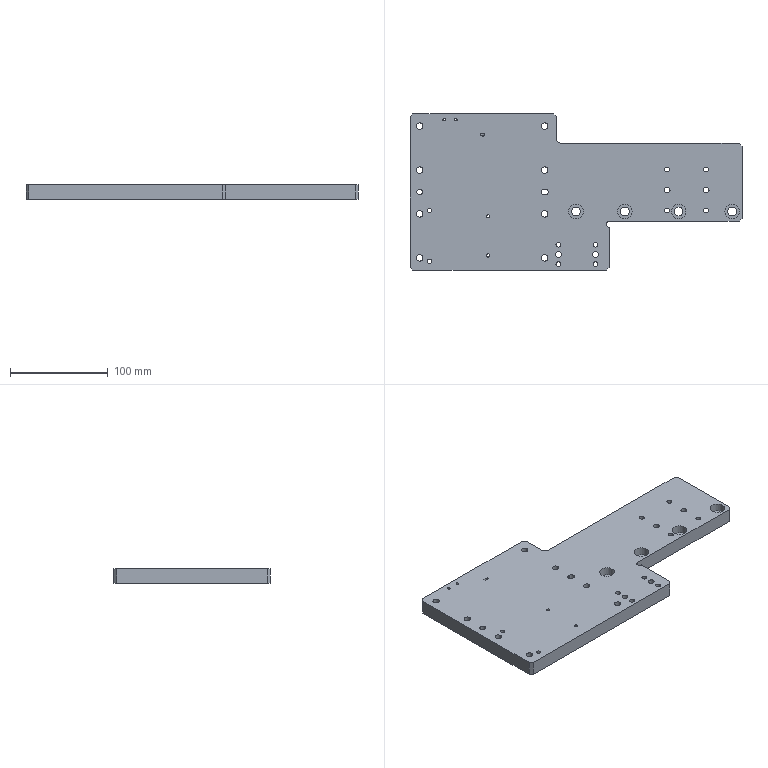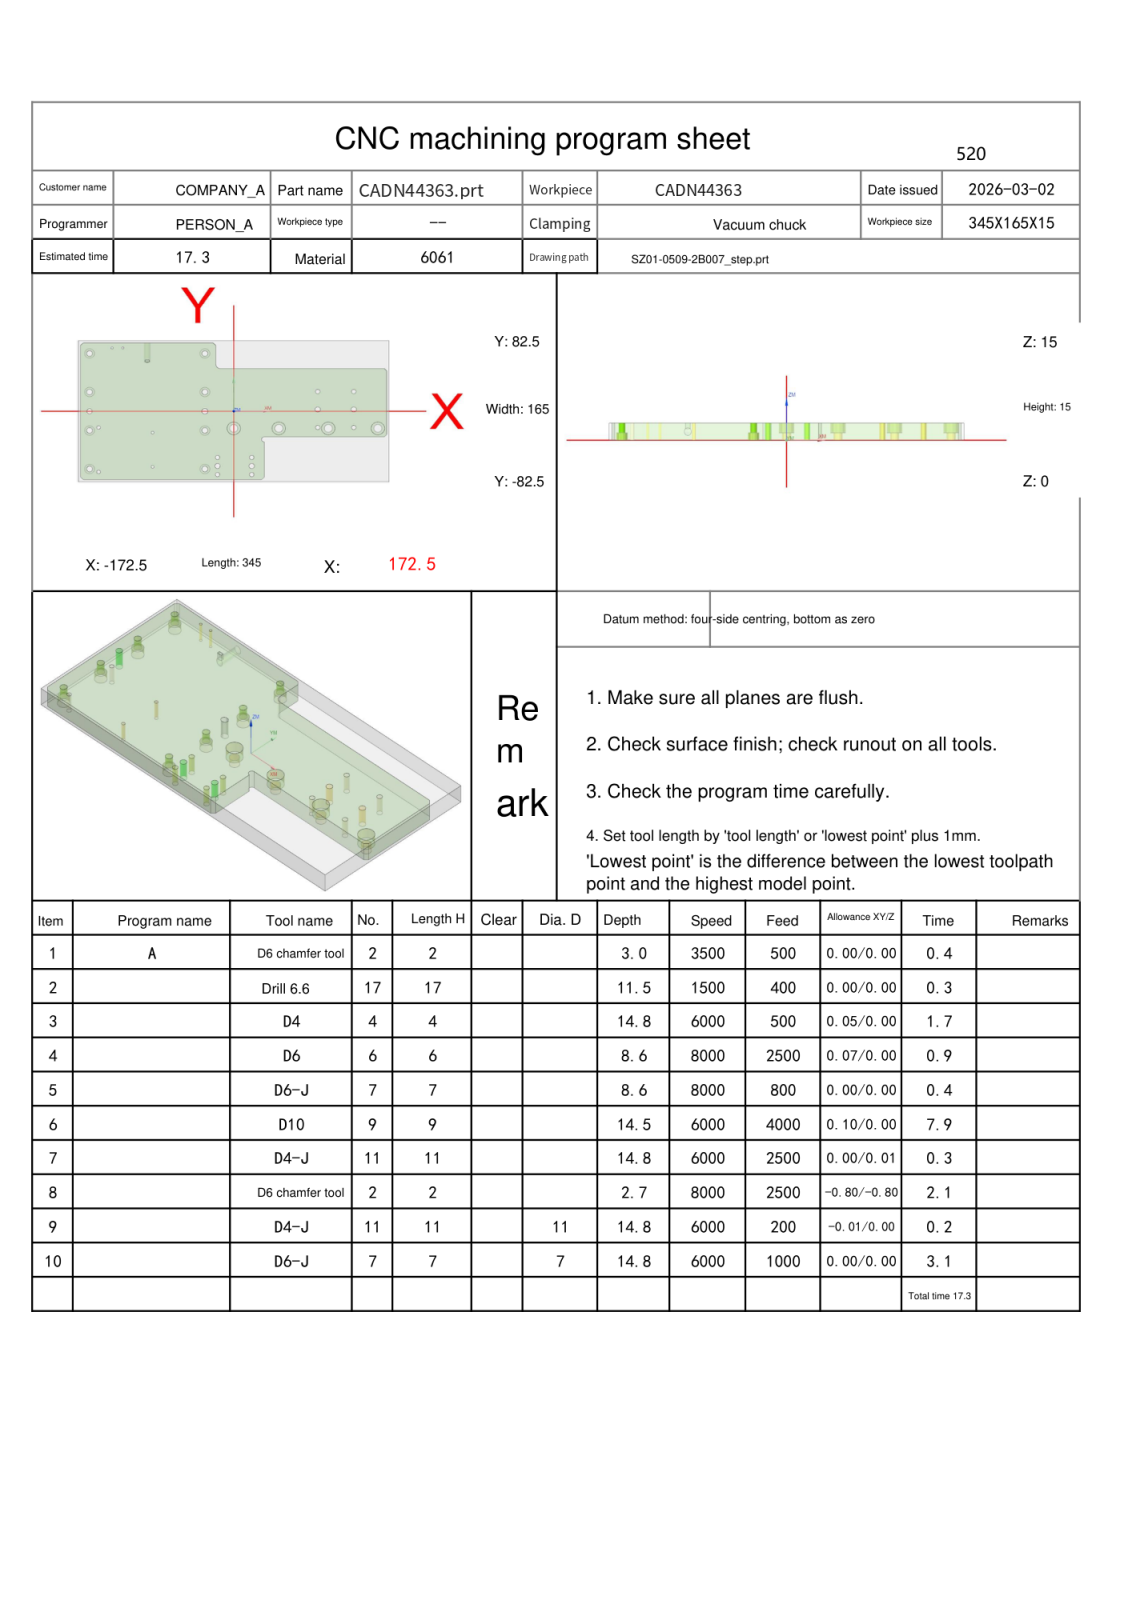NC program | NX | posted by the shop | part box 340 x 160 x 15 mm
Lines 1 to 977 of 3961:
%
O0001
(Machine time: 19.14 MIN)
(===Total Tool:7===)
(T2=D6 chamfer tool   D=6.   R=0.   D-  H02 Z=12.   )
(T17=drill 6.6  D=6.6  DR_a=120 D-  H17 Z=3.49  )
(T4=D4      D=4.   R=0.   D-  H04 Z=0.2   )
(T6=D6      D=6.   R=0.   D-  H06 Z=6.4   )
(T7=D6-J    D=6.   R=0.   D-  H07 Z=0.2   )
(T9=D10     D=10.  R=0.   D-  H09 Z=0.5   )
(T11=D4-J   D=4.   R=0.   D-  H11 Z=0.2   )
G80 G90 G17 G49 G40
G91 G28 Z0
M01
N1 T02 M06
(D6 chamfer tool D=6. R=0. H=02 ce=0.00 di=0.00)
G00 G90 G54 X93.275 Y23. M03 S3500
G43 H02 Z65.
M08
G98 G81 X93.275 Y23. Z12.9 R16. F500.
X133.275
Y-19.
X93.275
X20. Y-54.
Y-74.
X-18.
X-32. Y-67.5
X-18. Y-54.
X-32. Y-22.5
Y22.5
Y67.5
X-90. Y-25.
Y-65.
X-150. Y-71.
X-160. Y-67.5
Y-22.5
X-150. Y-19.
X-160. Y22.5
Y67.5
G80
G00 Z65.
G00 G90 X-135. Y74. M03 S3500
Z65.
G98 G81 X-135. Y74. Z13.5 R16. F500.
X-123.
G80
G00 Z65.
G00 G90 X-160. Y0.0 M03 S3500
Z65.
G98 G81 X-160. Y0.0 Z12. R16. F500.
X-18. Y-64.
X20.
X93.275 Y2.
X133.275
G80
G00 Z65.
G00 G90 X0.0 Y-20. M03 S3500
Z65.
G98 G81 X0.0 Y-20. Z13.5 R16. F500.
X50.
X105.
X160.
G80
G00 Z65.
G91 G28 Z0.0
M05
M09
G91 G28 Z0.0
M01
N2 T17 M06
(drill 6.6 D=6.6 DR_a=120 H=17)
G00 G90 G54 X-160. Y-67.5 M03 S1500
G43 H17 Z65.
M08
G98 G83 X-160. Y-67.5 Z3.495 R16. F400. Q5.
Y-22.5
Y22.5
Y67.5
X-32.
Y22.5
Y-22.5
Y-67.5
G80
G00 Z65.
G91 G28 Z0.0
M05
M09
G91 G28 Z0.0
M01
N3 T04 M06
(D4  D=4. R=0. H=04 ce=0.05 di=0.00)
G00 G90 G54 X-32. Y-.95 M03 S6000
G43 H04 Z65.
M08
Z15.5
G01 X-31.5 Z15.491 F500.
G03 X-30.55 Y0.0 Z15.463 I0.0 J.95
X-31.5 Y.95 Z15.435 I-.95 J0.0
G01 X-32.5 Z15.416
G03 X-33.45 Y0.0 Z15.389 I0.0 J-.95
X-32.5 Y-.95 Z15.361 I.95 J0.0
G01 X-31.5 Z15.342
G03 X-30.55 Y0.0 Z15.314 I0.0 J.95
X-31.5 Y.95 Z15.287 I-.95 J0.0
G01 X-32.5 Z15.268
G03 X-33.45 Y0.0 Z15.24 I0.0 J-.95
X-32.5 Y-.95 Z15.212 I.95 J0.0
G01 X-31.5 Z15.194
G03 X-30.55 Y0.0 Z15.166 I0.0 J.95
X-31.5 Y.95 Z15.138 I-.95 J0.0
G01 X-32.5 Z15.119
G03 X-33.45 Y0.0 Z15.092 I0.0 J-.95
X-32.5 Y-.95 Z15.064 I.95 J0.0
G01 X-31.5 Z15.045
G03 X-30.55 Y0.0 Z15.017 I0.0 J.95
X-31.5 Y.95 Z14.989 I-.95 J0.0
G01 X-32.5 Z14.971
G03 X-33.45 Y0.0 Z14.943 I0.0 J-.95
X-32.5 Y-.95 Z14.915 I.95 J0.0
G01 X-31.5 Z14.897
G03 X-30.55 Y0.0 Z14.869 I0.0 J.95
X-31.5 Y.95 Z14.841 I-.95 J0.0
G01 X-32.5 Z14.822
G03 X-33.45 Y0.0 Z14.794 I0.0 J-.95
X-32.5 Y-.95 Z14.767 I.95 J0.0
G01 X-31.5 Z14.748
G03 X-30.55 Y0.0 Z14.72 I0.0 J.95
X-31.5 Y.95 Z14.692 I-.95 J0.0
G01 X-32.5 Z14.674
G03 X-33.45 Y0.0 Z14.646 I0.0 J-.95
X-32.5 Y-.95 Z14.618 I.95 J0.0
G01 X-31.5 Z14.599
G03 X-30.55 Y0.0 Z14.572 I0.0 J.95
X-31.5 Y.95 Z14.544 I-.95 J0.0
G01 X-32.5 Z14.525
G03 X-33.45 Y0.0 Z14.497 I0.0 J-.95
X-32.5 Y-.95 Z14.47 I.95 J0.0
G01 X-31.5 Z14.451
G03 X-30.55 Y0.0 Z14.423 I0.0 J.95
X-31.5 Y.95 Z14.395 I-.95 J0.0
G01 X-32.5 Z14.377
G03 X-33.45 Y0.0 Z14.349 I0.0 J-.95
X-32.5 Y-.95 Z14.321 I.95 J0.0
G01 X-31.5 Z14.302
G03 X-30.55 Y0.0 Z14.275 I0.0 J.95
X-31.5 Y.95 Z14.247 I-.95 J0.0
G01 X-32.5 Z14.228
G03 X-33.45 Y0.0 Z14.2 I0.0 J-.95
X-32.5 Y-.95 Z14.172 I.95 J0.0
G01 X-31.5 Z14.154
G03 X-30.55 Y0.0 Z14.126 I0.0 J.95
X-31.5 Y.95 Z14.098 I-.95 J0.0
G01 X-32.5 Z14.08
G03 X-33.45 Y0.0 Z14.052 I0.0 J-.95
X-32.5 Y-.95 Z14.024 I.95 J0.0
G01 X-31.5 Z14.005
G03 X-30.55 Y0.0 Z13.977 I0.0 J.95
X-31.5 Y.95 Z13.95 I-.95 J0.0
G01 X-32.5 Z13.931
G03 X-33.45 Y0.0 Z13.903 I0.0 J-.95
X-32.5 Y-.95 Z13.875 I.95 J0.0
G01 X-31.5 Z13.857
G03 X-30.55 Y0.0 Z13.829 I0.0 J.95
X-31.5 Y.95 Z13.801 I-.95 J0.0
G01 X-32.5 Z13.782
G03 X-33.45 Y0.0 Z13.755 I0.0 J-.95
X-32.5 Y-.95 Z13.727 I.95 J0.0
G01 X-31.5 Z13.708
G03 X-30.55 Y0.0 Z13.68 I0.0 J.95
X-31.5 Y.95 Z13.653 I-.95 J0.0
G01 X-32.5 Z13.634
G03 X-33.45 Y0.0 Z13.606 I0.0 J-.95
X-32.5 Y-.95 Z13.578 I.95 J0.0
G01 X-31.5 Z13.56
G03 X-30.55 Y0.0 Z13.532 I0.0 J.95
X-31.5 Y.95 Z13.504 I-.95 J0.0
G01 X-32.5 Z13.485
G03 X-33.45 Y0.0 Z13.458 I0.0 J-.95
X-32.5 Y-.95 Z13.43 I.95 J0.0
G01 X-31.5 Z13.411
G03 X-30.55 Y0.0 Z13.383 I0.0 J.95
X-31.5 Y.95 Z13.355 I-.95 J0.0
G01 X-32.5 Z13.337
G03 X-33.45 Y0.0 Z13.309 I0.0 J-.95
X-32.5 Y-.95 Z13.281 I.95 J0.0
G01 X-31.5 Z13.263
G03 X-30.55 Y0.0 Z13.235 I0.0 J.95
X-31.5 Y.95 Z13.207 I-.95 J0.0
G01 X-32.5 Z13.188
G03 X-33.45 Y0.0 Z13.16 I0.0 J-.95
X-32.5 Y-.95 Z13.133 I.95 J0.0
G01 X-31.5 Z13.114
G03 X-30.55 Y0.0 Z13.086 I0.0 J.95
X-31.5 Y.95 Z13.058 I-.95 J0.0
G01 X-32.5 Z13.04
G03 X-33.45 Y0.0 Z13.012 I0.0 J-.95
X-32.5 Y-.95 Z12.984 I.95 J0.0
G01 X-31.5 Z12.965
G03 X-30.55 Y0.0 Z12.938 I0.0 J.95
X-31.5 Y.95 Z12.91 I-.95 J0.0
G01 X-32.5 Z12.891
G03 X-33.45 Y0.0 Z12.863 I0.0 J-.95
X-32.5 Y-.95 Z12.836 I.95 J0.0
G01 X-31.5 Z12.817
G03 X-30.55 Y0.0 Z12.789 I0.0 J.95
X-31.5 Y.95 Z12.761 I-.95 J0.0
G01 X-32.5 Z12.743
G03 X-33.45 Y0.0 Z12.715 I0.0 J-.95
X-32.5 Y-.95 Z12.687 I.95 J0.0
G01 X-31.5 Z12.668
G03 X-30.55 Y0.0 Z12.641 I0.0 J.95
X-31.5 Y.95 Z12.613 I-.95 J0.0
G01 X-32.5 Z12.594
G03 X-33.45 Y0.0 Z12.566 I0.0 J-.95
X-32.5 Y-.95 Z12.538 I.95 J0.0
G01 X-31.5 Z12.52
G03 X-30.55 Y0.0 Z12.492 I0.0 J.95
X-31.5 Y.95 Z12.464 I-.95 J0.0
G01 X-32.5 Z12.446
G03 X-33.45 Y0.0 Z12.418 I0.0 J-.95
X-32.5 Y-.95 Z12.39 I.95 J0.0
G01 X-31.5 Z12.371
G03 X-30.55 Y0.0 Z12.343 I0.0 J.95
X-31.5 Y.95 Z12.316 I-.95 J0.0
G01 X-32.5 Z12.297
G03 X-33.45 Y0.0 Z12.269 I0.0 J-.95
X-32.5 Y-.95 Z12.241 I.95 J0.0
G01 X-31.5 Z12.223
G03 X-30.55 Y0.0 Z12.195 I0.0 J.95
X-31.5 Y.95 Z12.167 I-.95 J0.0
G01 X-32.5 Z12.148
G03 X-33.45 Y0.0 Z12.121 I0.0 J-.95
X-32.5 Y-.95 Z12.093 I.95 J0.0
G01 X-31.5 Z12.074
G03 X-30.55 Y0.0 Z12.046 I0.0 J.95
X-31.5 Y.95 Z12.019 I-.95 J0.0
G01 X-32.5 Z12.
G03 X-33.45 Y0.0 Z11.972 I0.0 J-.95
X-32.5 Y-.95 Z11.944 I.95 J0.0
G01 X-31.5 Z11.926
G03 X-30.55 Y0.0 Z11.898 I0.0 J.95
X-31.5 Y.95 Z11.87 I-.95 J0.0
G01 X-32.5 Z11.851
G03 X-33.45 Y0.0 Z11.824 I0.0 J-.95
X-32.5 Y-.95 Z11.796 I.95 J0.0
G01 X-31.5 Z11.777
G03 X-30.55 Y0.0 Z11.749 I0.0 J.95
X-31.5 Y.95 Z11.721 I-.95 J0.0
G01 X-32.5 Z11.703
G03 X-33.45 Y0.0 Z11.675 I0.0 J-.95
X-32.5 Y-.95 Z11.647 I.95 J0.0
G01 X-31.5 Z11.629
G03 X-30.55 Y0.0 Z11.601 I0.0 J.95
X-31.5 Y.95 Z11.573 I-.95 J0.0
G01 X-32.5 Z11.554
G03 X-33.45 Y0.0 Z11.526 I0.0 J-.95
X-32.5 Y-.95 Z11.499 I.95 J0.0
G01 X-31.5 Z11.48
G03 X-30.55 Y0.0 Z11.452 I0.0 J.95
X-31.5 Y.95 Z11.424 I-.95 J0.0
G01 X-32.5 Z11.406
G03 X-33.45 Y0.0 Z11.378 I0.0 J-.95
X-32.5 Y-.95 Z11.35 I.95 J0.0
G01 X-31.5 Z11.331
G03 X-30.55 Y0.0 Z11.304 I0.0 J.95
X-31.5 Y.95 Z11.276 I-.95 J0.0
G01 X-32.5 Z11.257
G03 X-33.45 Y0.0 Z11.229 I0.0 J-.95
X-32.5 Y-.95 Z11.202 I.95 J0.0
G01 X-31.5 Z11.183
G03 X-30.55 Y0.0 Z11.155 I0.0 J.95
X-31.5 Y.95 Z11.127 I-.95 J0.0
G01 X-32.5 Z11.109
G03 X-33.45 Y0.0 Z11.081 I0.0 J-.95
X-32.5 Y-.95 Z11.053 I.95 J0.0
G01 X-31.5 Z11.034
G03 X-30.55 Y0.0 Z11.007 I0.0 J.95
X-31.5 Y.95 Z10.979 I-.95 J0.0
G01 X-32.5 Z10.96
G03 X-33.45 Y0.0 Z10.932 I0.0 J-.95
X-32.5 Y-.95 Z10.904 I.95 J0.0
G01 X-31.5 Z10.886
G03 X-30.55 Y0.0 Z10.858 I0.0 J.95
X-31.5 Y.95 Z10.83 I-.95 J0.0
G01 X-32.5 Z10.812
G03 X-33.45 Y0.0 Z10.784 I0.0 J-.95
X-32.5 Y-.95 Z10.756 I.95 J0.0
G01 X-31.5 Z10.737
G03 X-30.55 Y0.0 Z10.709 I0.0 J.95
X-31.5 Y.95 Z10.682 I-.95 J0.0
G01 X-32.5 Z10.663
G03 X-33.45 Y0.0 Z10.635 I0.0 J-.95
X-32.5 Y-.95 Z10.607 I.95 J0.0
G01 X-31.5 Z10.589
G03 X-30.55 Y0.0 Z10.561 I0.0 J.95
X-31.5 Y.95 Z10.533 I-.95 J0.0
G01 X-32.5 Z10.514
G03 X-33.45 Y0.0 Z10.487 I0.0 J-.95
X-32.5 Y-.95 Z10.459 I.95 J0.0
G01 X-31.5 Z10.44
G03 X-30.55 Y0.0 Z10.412 I0.0 J.95
X-31.5 Y.95 Z10.385 I-.95 J0.0
G01 X-32.5 Z10.366
G03 X-33.45 Y0.0 Z10.338 I0.0 J-.95
X-32.5 Y-.95 Z10.31 I.95 J0.0
G01 X-31.5 Z10.292
G03 X-30.55 Y0.0 Z10.264 I0.0 J.95
X-31.5 Y.95 Z10.236 I-.95 J0.0
G01 X-32.5 Z10.217
G03 X-33.45 Y0.0 Z10.19 I0.0 J-.95
X-32.5 Y-.95 Z10.162 I.95 J0.0
G01 X-31.5 Z10.143
G03 X-30.55 Y0.0 Z10.115 I0.0 J.95
X-31.5 Y.95 Z10.087 I-.95 J0.0
G01 X-32.5 Z10.069
G03 X-33.45 Y0.0 Z10.041 I0.0 J-.95
X-32.5 Y-.95 Z10.013 I.95 J0.0
G01 X-31.5 Z9.995
G03 X-30.55 Y0.0 Z9.967 I0.0 J.95
X-31.5 Y.95 Z9.939 I-.95 J0.0
G01 X-32.5 Z9.92
G03 X-33.45 Y0.0 Z9.892 I0.0 J-.95
X-32.5 Y-.95 Z9.865 I.95 J0.0
G01 X-31.5 Z9.846
G03 X-30.55 Y0.0 Z9.818 I0.0 J.95
X-31.5 Y.95 Z9.79 I-.95 J0.0
G01 X-32.5 Z9.772
G03 X-33.45 Y0.0 Z9.744 I0.0 J-.95
X-32.5 Y-.95 Z9.716 I.95 J0.0
G01 X-31.5 Z9.697
G03 X-30.55 Y0.0 Z9.67 I0.0 J.95
X-31.5 Y.95 Z9.642 I-.95 J0.0
G01 X-32.5 Z9.623
G03 X-33.45 Y0.0 Z9.595 I0.0 J-.95
X-32.5 Y-.95 Z9.568 I.95 J0.0
G01 X-31.5 Z9.549
G03 X-30.55 Y0.0 Z9.521 I0.0 J.95
X-31.5 Y.95 Z9.493 I-.95 J0.0
G01 X-32.5 Z9.475
G03 X-33.45 Y0.0 Z9.447 I0.0 J-.95
X-32.5 Y-.95 Z9.419 I.95 J0.0
G01 X-31.5 Z9.4
G03 X-30.55 Y0.0 Z9.373 I0.0 J.95
X-31.5 Y.95 Z9.345 I-.95 J0.0
G01 X-32.5 Z9.326
G03 X-33.45 Y0.0 Z9.298 I0.0 J-.95
X-32.5 Y-.95 Z9.27 I.95 J0.0
G01 X-31.5 Z9.252
G03 X-30.55 Y0.0 Z9.224 I0.0 J.95
X-31.5 Y.95 Z9.196 I-.95 J0.0
G01 X-32.5 Z9.178
G03 X-33.45 Y0.0 Z9.15 I0.0 J-.95
X-32.5 Y-.95 Z9.122 I.95 J0.0
G01 X-31.5 Z9.103
G03 X-30.55 Y0.0 Z9.075 I0.0 J.95
X-31.5 Y.95 Z9.048 I-.95 J0.0
G01 X-32.5 Z9.029
G03 X-33.45 Y0.0 Z9.001 I0.0 J-.95
X-32.5 Y-.95 Z8.973 I.95 J0.0
G01 X-31.5 Z8.955
G03 X-30.55 Y0.0 Z8.927 I0.0 J.95
X-31.5 Y.95 Z8.899 I-.95 J0.0
G01 X-32.5 Z8.88
G03 X-33.45 Y0.0 Z8.853 I0.0 J-.95
X-32.5 Y-.95 Z8.825 I.95 J0.0
G01 X-31.5 Z8.806
G03 X-30.55 Y0.0 Z8.778 I0.0 J.95
X-31.5 Y.95 Z8.751 I-.95 J0.0
G01 X-32.5 Z8.732
G03 X-33.45 Y0.0 Z8.704 I0.0 J-.95
X-32.5 Y-.95 Z8.676 I.95 J0.0
G01 X-31.5 Z8.658
G03 X-30.55 Y0.0 Z8.63 I0.0 J.95
X-31.5 Y.95 Z8.602 I-.95 J0.0
G01 X-32.5 Z8.583
G03 X-33.45 Y0.0 Z8.556 I0.0 J-.95
X-32.5 Y-.95 Z8.528 I.95 J0.0
G01 X-31.5 Z8.509
G03 X-30.55 Y0.0 Z8.481 I0.0 J.95
X-31.5 Y.95 Z8.453 I-.95 J0.0
G01 X-32.5 Z8.435
G03 X-33.45 Y0.0 Z8.407 I0.0 J-.95
X-32.5 Y-.95 Z8.379 I.95 J0.0
G01 X-31.5 Z8.361
G03 X-30.55 Y0.0 Z8.333 I0.0 J.95
X-31.5 Y.95 Z8.305 I-.95 J0.0
G01 X-32.5 Z8.286
G03 X-33.45 Y0.0 Z8.258 I0.0 J-.95
X-32.5 Y-.95 Z8.231 I.95 J0.0
G01 X-31.5 Z8.212
G03 X-30.55 Y0.0 Z8.184 I0.0 J.95
X-31.5 Y.95 Z8.156 I-.95 J0.0
G01 X-32.5 Z8.138
G03 X-33.45 Y0.0 Z8.11 I0.0 J-.95
X-32.5 Y-.95 Z8.082 I.95 J0.0
G01 X-31.5 Z8.063
G03 X-30.55 Y0.0 Z8.036 I0.0 J.95
X-31.5 Y.95 Z8.008 I-.95 J0.0
G01 X-32.5 Z7.989
G03 X-33.45 Y0.0 Z7.961 I0.0 J-.95
X-32.5 Y-.95 Z7.934 I.95 J0.0
G01 X-31.5 Z7.915
G03 X-30.55 Y0.0 Z7.887 I0.0 J.95
X-31.5 Y.95 Z7.859 I-.95 J0.0
G01 X-32.5 Z7.841
G03 X-33.45 Y0.0 Z7.813 I0.0 J-.95
X-32.5 Y-.95 Z7.785 I.95 J0.0
G01 X-31.5 Z7.766
G03 X-30.55 Y0.0 Z7.739 I0.0 J.95
X-31.5 Y.95 Z7.711 I-.95 J0.0
G01 X-32.5 Z7.692
G03 X-33.45 Y0.0 Z7.664 I0.0 J-.95
X-32.5 Y-.95 Z7.637 I.95 J0.0
G01 X-31.5 Z7.618
G03 X-30.55 Y0.0 Z7.59 I0.0 J.95
X-31.5 Y.95 Z7.562 I-.95 J0.0
G01 X-32.5 Z7.544
G03 X-33.45 Y0.0 Z7.516 I0.0 J-.95
X-32.5 Y-.95 Z7.488 I.95 J0.0
G01 X-31.5 Z7.469
G03 X-30.55 Y0.0 Z7.442 I0.0 J.95
X-31.5 Y.95 Z7.414 I-.95 J0.0
G01 X-32.5 Z7.395
G03 X-33.45 Y0.0 Z7.367 I0.0 J-.95
X-32.5 Y-.95 Z7.339 I.95 J0.0
G01 X-31.5 Z7.321
G03 X-30.55 Y0.0 Z7.293 I0.0 J.95
X-31.5 Y.95 Z7.265 I-.95 J0.0
G01 X-32.5 Z7.247
G03 X-33.45 Y0.0 Z7.219 I0.0 J-.95
X-32.5 Y-.95 Z7.191 I.95 J0.0
G01 X-31.5 Z7.172
G03 X-30.55 Y0.0 Z7.144 I0.0 J.95
X-31.5 Y.95 Z7.117 I-.95 J0.0
G01 X-32.5 Z7.098
G03 X-33.45 Y0.0 Z7.07 I0.0 J-.95
X-32.5 Y-.95 Z7.042 I.95 J0.0
G01 X-31.5 Z7.024
G03 X-30.55 Y0.0 Z6.996 I0.0 J.95
X-31.5 Y.95 Z6.968 I-.95 J0.0
G01 X-32.5 Z6.949
G03 X-33.45 Y0.0 Z6.922 I0.0 J-.95
X-32.5 Y-.95 Z6.894 I.95 J0.0
G01 X-31.5 Z6.875
G03 X-30.55 Y0.0 Z6.847 I0.0 J.95
X-31.5 Y.95 Z6.82 I-.95 J0.0
G01 X-32.5 Z6.801
G03 X-33.45 Y0.0 Z6.773 I0.0 J-.95
X-32.5 Y-.95 Z6.745 I.95 J0.0
G01 X-31.5 Z6.727
G03 X-30.55 Y0.0 Z6.699 I0.0 J.95
X-31.5 Y.95 Z6.671 I-.95 J0.0
G01 X-32.5 Z6.652
G03 X-33.45 Y0.0 Z6.625 I0.0 J-.95
X-32.5 Y-.95 Z6.597 I.95 J0.0
G01 X-31.5 Z6.578
G03 X-30.55 Y0.0 Z6.55 I0.0 J.95
X-31.5 Y.95 Z6.522 I-.95 J0.0
G01 X-32.5 Z6.504
G03 X-33.45 Y0.0 Z6.476 I0.0 J-.95
X-32.5 Y-.95 Z6.448 I.95 J0.0
G01 X-31.5 Z6.43
G03 X-30.55 Y0.0 Z6.402 I0.0 J.95
X-31.5 Y.95 Z6.374 I-.95 J0.0
G01 X-32.5 Z6.355
G03 X-33.45 Y0.0 Z6.327 I0.0 J-.95
X-32.5 Y-.95 Z6.3 I.95 J0.0
G01 X-31.5 Z6.281
G03 X-30.55 Y0.0 Z6.253 I0.0 J.95
X-31.5 Y.95 Z6.225 I-.95 J0.0
G01 X-32.5 Z6.207
G03 X-33.45 Y0.0 Z6.179 I0.0 J-.95
X-32.5 Y-.95 Z6.151 I.95 J0.0
G01 X-31.5 Z6.132
G03 X-30.55 Y0.0 Z6.105 I0.0 J.95
X-31.5 Y.95 Z6.077 I-.95 J0.0
G01 X-32.5 Z6.058
G03 X-33.45 Y0.0 Z6.03 I0.0 J-.95
X-32.5 Y-.95 Z6.003 I.95 J0.0
G01 X-31.5 Z5.984
G03 X-30.55 Y0.0 Z5.956 I0.0 J.95
X-31.5 Y.95 Z5.928 I-.95 J0.0
G01 X-32.5 Z5.91
G03 X-33.45 Y0.0 Z5.882 I0.0 J-.95
X-32.5 Y-.95 Z5.854 I.95 J0.0
G01 X-31.5 Z5.835
G03 X-30.55 Y0.0 Z5.808 I0.0 J.95
X-31.5 Y.95 Z5.78 I-.95 J0.0
G01 X-32.5 Z5.761
G03 X-33.45 Y0.0 Z5.733 I0.0 J-.95
X-32.5 Y-.95 Z5.705 I.95 J0.0
G01 X-31.5 Z5.687
G03 X-30.55 Y0.0 Z5.659 I0.0 J.95
X-31.5 Y.95 Z5.631 I-.95 J0.0
G01 X-32.5 Z5.613
G03 X-33.45 Y0.0 Z5.585 I0.0 J-.95
X-32.5 Y-.95 Z5.557 I.95 J0.0
G01 X-31.5 Z5.538
G03 X-30.55 Y0.0 Z5.51 I0.0 J.95
X-31.5 Y.95 Z5.483 I-.95 J0.0
G01 X-32.5 Z5.464
G03 X-33.45 Y0.0 Z5.436 I0.0 J-.95
X-32.5 Y-.95 Z5.408 I.95 J0.0
G01 X-31.5 Z5.39
G03 X-30.55 Y0.0 Z5.362 I0.0 J.95
X-31.5 Y.95 Z5.334 I-.95 J0.0
G01 X-32.5 Z5.315
G03 X-33.45 Y0.0 Z5.288 I0.0 J-.95
X-32.5 Y-.95 Z5.26 I.95 J0.0
G01 X-31.5 Z5.241
G03 X-30.55 Y0.0 Z5.213 I0.0 J.95
X-31.5 Y.95 Z5.186 I-.95 J0.0
G01 X-32.5 Z5.167
G03 X-33.45 Y0.0 Z5.139 I0.0 J-.95
X-32.5 Y-.95 Z5.111 I.95 J0.0
G01 X-31.5 Z5.093
G03 X-30.55 Y0.0 Z5.065 I0.0 J.95
X-31.5 Y.95 Z5.037 I-.95 J0.0
G01 X-32.5 Z5.018
G03 X-33.45 Y0.0 Z4.991 I0.0 J-.95
X-32.5 Y-.95 Z4.963 I.95 J0.0
G01 X-31.5 Z4.944
G03 X-30.55 Y0.0 Z4.916 I0.0 J.95
X-31.5 Y.95 Z4.888 I-.95 J0.0
G01 X-32.5 Z4.87
G03 X-33.45 Y0.0 Z4.842 I0.0 J-.95
X-32.5 Y-.95 Z4.814 I.95 J0.0
G01 X-31.5 Z4.796
G03 X-30.55 Y0.0 Z4.768 I0.0 J.95
X-31.5 Y.95 Z4.74 I-.95 J0.0
G01 X-32.5 Z4.721
G03 X-33.45 Y0.0 Z4.693 I0.0 J-.95
X-32.5 Y-.95 Z4.666 I.95 J0.0
G01 X-31.5 Z4.647
G03 X-30.55 Y0.0 Z4.619 I0.0 J.95
X-31.5 Y.95 Z4.591 I-.95 J0.0
G01 X-32.5 Z4.573
G03 X-33.45 Y0.0 Z4.545 I0.0 J-.95
X-32.5 Y-.95 Z4.517 I.95 J0.0
G01 X-31.5 Z4.498
G03 X-30.55 Y0.0 Z4.471 I0.0 J.95
X-31.5 Y.95 Z4.443 I-.95 J0.0
G01 X-32.5 Z4.424
G03 X-33.45 Y0.0 Z4.396 I0.0 J-.95
X-32.5 Y-.95 Z4.369 I.95 J0.0
G01 X-31.5 Z4.35
G03 X-30.55 Y0.0 Z4.322 I0.0 J.95
X-31.5 Y.95 Z4.294 I-.95 J0.0
G01 X-32.5 Z4.276
G03 X-33.45 Y0.0 Z4.248 I0.0 J-.95
X-32.5 Y-.95 Z4.22 I.95 J0.0
G01 X-31.5 Z4.201
G03 X-30.55 Y0.0 Z4.174 I0.0 J.95
X-31.5 Y.95 Z4.146 I-.95 J0.0
G01 X-32.5 Z4.127
G03 X-33.45 Y0.0 Z4.099 I0.0 J-.95
X-32.5 Y-.95 Z4.071 I.95 J0.0
G01 X-31.5 Z4.053
G03 X-30.55 Y0.0 Z4.025 I0.0 J.95
X-31.5 Y.95 Z3.997 I-.95 J0.0
G01 X-32.5 Z3.979
G03 X-33.45 Y0.0 Z3.951 I0.0 J-.95
X-32.5 Y-.95 Z3.923 I.95 J0.0
G01 X-31.5 Z3.904
G03 X-30.55 Y0.0 Z3.876 I0.0 J.95
X-31.5 Y.95 Z3.849 I-.95 J0.0
G01 X-32.5 Z3.83
G03 X-33.45 Y0.0 Z3.802 I0.0 J-.95
X-32.5 Y-.95 Z3.774 I.95 J0.0
G01 X-31.5 Z3.756
G03 X-30.55 Y0.0 Z3.728 I0.0 J.95
X-31.5 Y.95 Z3.7 I-.95 J0.0
G01 X-32.5 Z3.681
G03 X-33.45 Y0.0 Z3.654 I0.0 J-.95
X-32.5 Y-.95 Z3.626 I.95 J0.0
G01 X-31.5 Z3.607
G03 X-30.55 Y0.0 Z3.579 I0.0 J.95
X-31.5 Y.95 Z3.552 I-.95 J0.0
G01 X-32.5 Z3.533
G03 X-33.45 Y0.0 Z3.505 I0.0 J-.95
X-32.5 Y-.95 Z3.477 I.95 J0.0
G01 X-31.5 Z3.459
G03 X-30.55 Y0.0 Z3.431 I0.0 J.95
X-31.5 Y.95 Z3.403 I-.95 J0.0
G01 X-32.5 Z3.384
G03 X-33.45 Y0.0 Z3.357 I0.0 J-.95
X-32.5 Y-.95 Z3.329 I.95 J0.0
G01 X-31.5 Z3.31
G03 X-30.55 Y0.0 Z3.282 I0.0 J.95
X-31.5 Y.95 Z3.254 I-.95 J0.0
G01 X-32.5 Z3.236
G03 X-33.45 Y0.0 Z3.208 I0.0 J-.95
X-32.5 Y-.95 Z3.18 I.95 J0.0
G01 X-31.5 Z3.162
G03 X-30.55 Y0.0 Z3.134 I0.0 J.95
X-31.5 Y.95 Z3.106 I-.95 J0.0
G01 X-32.5 Z3.087
G03 X-33.45 Y0.0 Z3.059 I0.0 J-.95
X-32.5 Y-.95 Z3.032 I.95 J0.0
G01 X-31.5 Z3.013
G03 X-30.55 Y0.0 Z2.985 I0.0 J.95
X-31.5 Y.95 Z2.957 I-.95 J0.0
G01 X-32.5 Z2.939
G03 X-33.45 Y0.0 Z2.911 I0.0 J-.95
X-32.5 Y-.95 Z2.883 I.95 J0.0
G01 X-31.5 Z2.864
G03 X-30.55 Y0.0 Z2.837 I0.0 J.95
X-31.5 Y.95 Z2.809 I-.95 J0.0
G01 X-32.5 Z2.79
G03 X-33.45 Y0.0 Z2.762 I0.0 J-.95
X-32.5 Y-.95 Z2.735 I.95 J0.0
G01 X-31.5 Z2.716
G03 X-30.55 Y0.0 Z2.688 I0.0 J.95
X-31.5 Y.95 Z2.66 I-.95 J0.0
G01 X-32.5 Z2.642
G03 X-33.45 Y0.0 Z2.614 I0.0 J-.95
X-32.5 Y-.95 Z2.586 I.95 J0.0
G01 X-31.5 Z2.567
G03 X-30.55 Y0.0 Z2.54 I0.0 J.95
X-31.5 Y.95 Z2.512 I-.95 J0.0
G01 X-32.5 Z2.493
G03 X-33.45 Y0.0 Z2.465 I0.0 J-.95
X-32.5 Y-.95 Z2.437 I.95 J0.0
G01 X-31.5 Z2.419
G03 X-30.55 Y0.0 Z2.391 I0.0 J.95
X-31.5 Y.95 Z2.363 I-.95 J0.0
G01 X-32.5 Z2.345
G03 X-33.45 Y0.0 Z2.317 I0.0 J-.95
X-32.5 Y-.95 Z2.289 I.95 J0.0
G01 X-31.5 Z2.27
G03 X-30.55 Y0.0 Z2.242 I0.0 J.95
X-31.5 Y.95 Z2.215 I-.95 J0.0
G01 X-32.5 Z2.196
G03 X-33.45 Y0.0 Z2.168 I0.0 J-.95
X-32.5 Y-.95 Z2.14 I.95 J0.0
G01 X-31.5 Z2.122
G03 X-30.55 Y0.0 Z2.094 I0.0 J.95
X-31.5 Y.95 Z2.066 I-.95 J0.0
G01 X-32.5 Z2.047
G03 X-33.45 Y0.0 Z2.02 I0.0 J-.95
X-32.5 Y-.95 Z1.992 I.95 J0.0
G01 X-31.5 Z1.973
G03 X-30.55 Y0.0 Z1.945 I0.0 J.95
X-31.5 Y.95 Z1.918 I-.95 J0.0
G01 X-32.5 Z1.899
G03 X-33.45 Y0.0 Z1.871 I0.0 J-.95
X-32.5 Y-.95 Z1.843 I.95 J0.0
G01 X-31.5 Z1.825
G03 X-30.55 Y0.0 Z1.797 I0.0 J.95
X-31.5 Y.95 Z1.769 I-.95 J0.0
G01 X-32.5 Z1.75
G03 X-33.45 Y0.0 Z1.723 I0.0 J-.95
X-32.5 Y-.95 Z1.695 I.95 J0.0
G01 X-31.5 Z1.676
G03 X-30.55 Y0.0 Z1.648 I0.0 J.95
X-31.5 Y.95 Z1.62 I-.95 J0.0
G01 X-32.5 Z1.602
G03 X-33.45 Y0.0 Z1.574 I0.0 J-.95
X-32.5 Y-.95 Z1.546 I.95 J0.0
G01 X-31.5 Z1.528
G03 X-30.55 Y0.0 Z1.5 I0.0 J.95
X-31.5 Y.95 Z1.472 I-.95 J0.0
G01 X-32.5 Z1.453
G03 X-33.45 Y0.0 Z1.425 I0.0 J-.95
X-32.5 Y-.95 Z1.398 I.95 J0.0
G01 X-31.5 Z1.379
G03 X-30.55 Y0.0 Z1.351 I0.0 J.95
X-31.5 Y.95 Z1.323 I-.95 J0.0
G01 X-32.5 Z1.305
G03 X-33.45 Y0.0 Z1.277 I0.0 J-.95
X-32.5 Y-.95 Z1.249 I.95 J0.0
G01 X-31.5 Z1.23
G03 X-30.55 Y0.0 Z1.203 I0.0 J.95
X-31.5 Y.95 Z1.175 I-.95 J0.0
G01 X-32.5 Z1.156
G03 X-33.45 Y0.0 Z1.128 I0.0 J-.95
X-32.5 Y-.95 Z1.101 I.95 J0.0
G01 X-31.5 Z1.082
G03 X-30.55 Y0.0 Z1.054 I0.0 J.95
X-31.5 Y.95 Z1.026 I-.95 J0.0
G01 X-32.5 Z1.008
G03 X-33.45 Y0.0 Z.98 I0.0 J-.95
X-32.5 Y-.95 Z.952 I.95 J0.0
G01 X-31.5 Z.933
G03 X-30.55 Y0.0 Z.906 I0.0 J.95
X-31.5 Y.95 Z.878 I-.95 J0.0
G01 X-32.5 Z.859
G03 X-33.45 Y0.0 Z.831 I0.0 J-.95
X-32.5 Y-.95 Z.803 I.95 J0.0
G01 X-31.5 Z.785
G03 X-30.55 Y0.0 Z.757 I0.0 J.95
X-31.5 Y.95 Z.729 I-.95 J0.0
G01 X-32.5 Z.711
G03 X-33.45 Y0.0 Z.683 I0.0 J-.95
X-32.5 Y-.95 Z.655 I.95 J0.0
G01 X-31.5 Z.636
G03 X-30.55 Y0.0 Z.608 I0.0 J.95
X-31.5 Y.95 Z.581 I-.95 J0.0
G01 X-32.5 Z.562
G03 X-33.45 Y0.0 Z.534 I0.0 J-.95
X-32.5 Y-.95 Z.506 I.95 J0.0
G01 X-31.5 Z.488
G03 X-30.55 Y0.0 Z.46 I0.0 J.95
X-31.5 Y.95 Z.432 I-.95 J0.0
G01 X-32.5 Z.413
G03 X-33.45 Y0.0 Z.386 I0.0 J-.95
X-32.5 Y-.95 Z.358 I.95 J0.0
G01 X-31.5 Z.339
G03 X-30.55 Y0.0 Z.311 I0.0 J.95
X-31.5 Y.95 Z.284 I-.95 J0.0
G01 X-32.5 Z.265
G03 X-33.45 Y0.0 Z.237 I0.0 J-.95
X-32.5 Y-.95 Z.209 I.95 J0.0
G01 X-32. Z.2
X-31.5
G03 X-30.55 Y0.0 I0.0 J.95
X-31.5 Y.95 I-.95 J0.0
G01 X-32.5
G03 X-33.45 Y0.0 I0.0 J-.95
X-32.5 Y-.95 I.95 J0.0
G01 X-32.
X-31.5
Z1.2
G00 Z65.
G91 G28 Z0.0
M05
M09
G91 G28 Z0.0
M01
N4 T06 M06
(D6  D=6. R=0. H=06 ce=0.07 di=0.00)
G00 G90 G54 X0.0 Y-20. M03 S8000
G43 H06 Z65.
M08
Z15.3
G03 X2.215 Y-22.215 I2.215 J0.0 F2500.
X4.43 Y-20. I0.0 J2.215
X4.43 Y-20. Z14.8 I-4.43 J0.0
X4.43 Y-20. Z14.3 I-4.43 J0.0
X4.43 Y-20. Z13.8 I-4.43 J0.0
X4.43 Y-20. Z13.3 I-4.43 J0.0
X4.43 Y-20. Z12.8 I-4.43 J0.0
X4.43 Y-20. Z12.3 I-4.43 J0.0
X4.43 Y-20. Z11.8 I-4.43 J0.0
X4.43 Y-20. Z11.3 I-4.43 J0.0
X4.43 Y-20. Z10.8 I-4.43 J0.0
X4.43 Y-20. Z10.3 I-4.43 J0.0
X4.43 Y-20. Z9.8 I-4.43 J0.0
X4.43 Y-20. Z9.3 I-4.43 J0.0
X4.43 Y-20. Z8.8 I-4.43 J0.0
X4.43 Y-20. Z8.3 I-4.43 J0.0
X4.43 Y-20. Z7.8 I-4.43 J0.0
X4.43 Y-20. Z7.3 I-4.43 J0.0
X4.43 Y-20. Z6.8 I-4.43 J0.0
X1.369 Y-24.213 Z6.4 I-4.43 J0.0
X4.43 Y-20. I-1.369 J4.213
X0.0 Y-15.57 I-4.43 J0.0
X-4.43 Y-20. I0.0 J-4.43
X0.0 Y-24.43 I4.43 J0.0
X1.369 Y-24.213 I0.0 J4.43
X2.899 Y-22.107 I-.684 J2.107
X.684 Y-19.892 I-2.215 J0.0
X0.0 Y-20. I0.0 J-2.215
G00 Z65.
X50.
Z15.3
G03 X52.215 Y-22.215 I2.215 J0.0
X54.43 Y-20. I0.0 J2.215
X54.43 Y-20. Z14.8 I-4.43 J0.0
X54.43 Y-20. Z14.3 I-4.43 J0.0
X54.43 Y-20. Z13.8 I-4.43 J0.0
X54.43 Y-20. Z13.3 I-4.43 J0.0
X54.43 Y-20. Z12.8 I-4.43 J0.0
X54.43 Y-20. Z12.3 I-4.43 J0.0
X54.43 Y-20. Z11.8 I-4.43 J0.0
X54.43 Y-20. Z11.3 I-4.43 J0.0
X54.43 Y-20. Z10.8 I-4.43 J0.0
X54.43 Y-20. Z10.3 I-4.43 J0.0
X54.43 Y-20. Z9.8 I-4.43 J0.0
X54.43 Y-20. Z9.3 I-4.43 J0.0
X54.43 Y-20. Z8.8 I-4.43 J0.0
X54.43 Y-20. Z8.3 I-4.43 J0.0
X54.43 Y-20. Z7.8 I-4.43 J0.0
X54.43 Y-20. Z7.3 I-4.43 J0.0
X54.43 Y-20. Z6.8 I-4.43 J0.0
X51.369 Y-24.213 Z6.4 I-4.43 J0.0
X54.43 Y-20. I-1.369 J4.213
X50. Y-15.57 I-4.43 J0.0
X45.57 Y-20. I0.0 J-4.43
X50. Y-24.43 I4.43 J0.0
X51.369 Y-24.213 I0.0 J4.43
X52.899 Y-22.107 I-.684 J2.107
X50.684 Y-19.892 I-2.215 J0.0
X50. Y-20. I0.0 J-2.215
G00 Z65.
X105.
Z15.3
G03 X107.215 Y-22.215 I2.215 J0.0
X109.43 Y-20. I0.0 J2.215
X109.43 Y-20. Z14.8 I-4.43 J0.0
X109.43 Y-20. Z14.3 I-4.43 J0.0
X109.43 Y-20. Z13.8 I-4.43 J0.0
X109.43 Y-20. Z13.3 I-4.43 J0.0
X109.43 Y-20. Z12.8 I-4.43 J0.0
X109.43 Y-20. Z12.3 I-4.43 J0.0
X109.43 Y-20. Z11.8 I-4.43 J0.0
X109.43 Y-20. Z11.3 I-4.43 J0.0
X109.43 Y-20. Z10.8 I-4.43 J0.0
X109.43 Y-20. Z10.3 I-4.43 J0.0
X109.43 Y-20. Z9.8 I-4.43 J0.0
X109.43 Y-20. Z9.3 I-4.43 J0.0
X109.43 Y-20. Z8.8 I-4.43 J0.0
X109.43 Y-20. Z8.3 I-4.43 J0.0
X109.43 Y-20. Z7.8 I-4.43 J0.0
X109.43 Y-20. Z7.3 I-4.43 J0.0
X109.43 Y-20. Z6.8 I-4.43 J0.0
X106.369 Y-24.213 Z6.4 I-4.43 J0.0
X109.43 Y-20. I-1.369 J4.213
X105. Y-15.57 I-4.43 J0.0
X100.57 Y-20. I0.0 J-4.43
X105. Y-24.43 I4.43 J0.0
X106.369 Y-24.213 I0.0 J4.43
X107.899 Y-22.107 I-.684 J2.107
X105.684 Y-19.892 I-2.215 J0.0
X105. Y-20. I0.0 J-2.215
G00 Z65.
X160.
Z15.3
G03 X162.215 Y-22.215 I2.215 J0.0
X164.43 Y-20. I0.0 J2.215
X164.43 Y-20. Z14.8 I-4.43 J0.0
X164.43 Y-20. Z14.3 I-4.43 J0.0
X164.43 Y-20. Z13.8 I-4.43 J0.0
X164.43 Y-20. Z13.3 I-4.43 J0.0
X164.43 Y-20. Z12.8 I-4.43 J0.0
X164.43 Y-20. Z12.3 I-4.43 J0.0
X164.43 Y-20. Z11.8 I-4.43 J0.0
X164.43 Y-20. Z11.3 I-4.43 J0.0
X164.43 Y-20. Z10.8 I-4.43 J0.0
X164.43 Y-20. Z10.3 I-4.43 J0.0
X164.43 Y-20. Z9.8 I-4.43 J0.0
X164.43 Y-20. Z9.3 I-4.43 J0.0
X164.43 Y-20. Z8.8 I-4.43 J0.0
X164.43 Y-20. Z8.3 I-4.43 J0.0
X164.43 Y-20. Z7.8 I-4.43 J0.0
X164.43 Y-20. Z7.3 I-4.43 J0.0
X164.43 Y-20. Z6.8 I-4.43 J0.0
X161.369 Y-24.213 Z6.4 I-4.43 J0.0
X164.43 Y-20. I-1.369 J4.213
X160. Y-15.57 I-4.43 J0.0
X155.57 Y-20. I0.0 J-4.43
X160. Y-24.43 I4.43 J0.0
X161.369 Y-24.213 I0.0 J4.43
X162.899 Y-22.107 I-.684 J2.107
X160.684 Y-19.892 I-2.215 J0.0
X160. Y-20. I0.0 J-2.215
G00 Z65.
G91 G28 Z0.0
M05
M09
G91 G28 Z0.0
M01
N5 T07 M06
(D6-J  D=6. R=0. H=07 ce=0.00 di=0.00)
G00 G90 G54 X0.0 Y-20. M03 S8000
G43 H07 Z65.
M08
Z10.7
G01 X4.115 Y-20.353 F800.
X4.145 Y-20.355
G03 X4.5 Y-20. I0.0 J.355
X0.0 Y-15.5 I-4.5 J0.0
X-4.5 Y-20. I0.0 J-4.5
X0.0 Y-24.5 I4.5 J0.0
X4.5 Y-20. I0.0 J4.5
X4.472 Y-19.501 I-4.5 J0.0
X4.12 Y-19.186 I-.353 J-.039
G01 X4.05 Y-19.192
X0.0 Y-20.
Z6.4 F10000.
X4.115 Y-20.353 F800.
X4.145 Y-20.355
G03 X4.5 Y-20. I0.0 J.355
X0.0 Y-15.5 I-4.5 J0.0
X-4.5 Y-20. I0.0 J-4.5
X0.0 Y-24.5 I4.5 J0.0
X4.5 Y-20. I0.0 J4.5
X4.472 Y-19.501 I-4.5 J0.0
X4.12 Y-19.186 I-.353 J-.039
G01 X4.05 Y-19.192
X0.0 Y-20.
G00 Z65.
X50.
Z10.7
G01 X54.115 Y-20.353
X54.145 Y-20.355
G03 X54.5 Y-20. I0.0 J.355
X50. Y-15.5 I-4.5 J0.0
X45.5 Y-20. I0.0 J-4.5
X50. Y-24.5 I4.5 J0.0
X54.5 Y-20. I0.0 J4.5
X54.472 Y-19.501 I-4.5 J0.0
X54.12 Y-19.186 I-.353 J-.039
G01 X54.05 Y-19.192
X50. Y-20.
Z6.4 F10000.
X54.115 Y-20.353 F800.
X54.145 Y-20.355
G03 X54.5 Y-20. I0.0 J.355
X50. Y-15.5 I-4.5 J0.0
X45.5 Y-20. I0.0 J-4.5
X50. Y-24.5 I4.5 J0.0
X54.5 Y-20. I0.0 J4.5
X54.472 Y-19.501 I-4.5 J0.0
X54.12 Y-19.186 I-.353 J-.039
G01 X54.05 Y-19.192
X50. Y-20.
G00 Z65.
X105.
Z10.7
G01 X109.115 Y-20.353
X109.145 Y-20.355
G03 X109.5 Y-20. I0.0 J.355
X105. Y-15.5 I-4.5 J0.0
X100.5 Y-20. I0.0 J-4.5
X105. Y-24.5 I4.5 J0.0
X109.5 Y-20. I0.0 J4.5
X109.472 Y-19.501 I-4.5 J0.0
X109.12 Y-19.186 I-.353 J-.039
G01 X109.05 Y-19.192
X105. Y-20.
Z6.4 F10000.
X109.115 Y-20.353 F800.
X109.145 Y-20.355
G03 X109.5 Y-20. I0.0 J.355
X105. Y-15.5 I-4.5 J0.0
X100.5 Y-20. I0.0 J-4.5
X105. Y-24.5 I4.5 J0.0
X109.5 Y-20. I0.0 J4.5
X109.472 Y-19.501 I-4.5 J0.0
X109.12 Y-19.186 I-.353 J-.039
G01 X109.05 Y-19.192
X105. Y-20.
G00 Z65.
X160.
Z10.7
G01 X164.115 Y-20.353
X164.145 Y-20.355
G03 X164.5 Y-20. I0.0 J.355
X160. Y-15.5 I-4.5 J0.0
X155.5 Y-20. I0.0 J-4.5
X160. Y-24.5 I4.5 J0.0
X164.5 Y-20. I0.0 J4.5
X164.472 Y-19.501 I-4.5 J0.0
X164.12 Y-19.186 I-.353 J-.039
G01 X164.05 Y-19.192
X160. Y-20.
Z6.4 F10000.
X164.115 Y-20.353 F800.
X164.145 Y-20.355
G03 X164.5 Y-20. I0.0 J.355
X160. Y-15.5 I-4.5 J0.0
X155.5 Y-20. I0.0 J-4.5
X160. Y-24.5 I4.5 J0.0
X164.5 Y-20. I0.0 J4.5
X164.472 Y-19.501 I-4.5 J0.0
X164.12 Y-19.186 I-.353 J-.039
G01 X164.05 Y-19.192
X160. Y-20.
G00 Z65.
G91 G28 Z0.0
M05
M09
G91 G28 Z0.0
M01